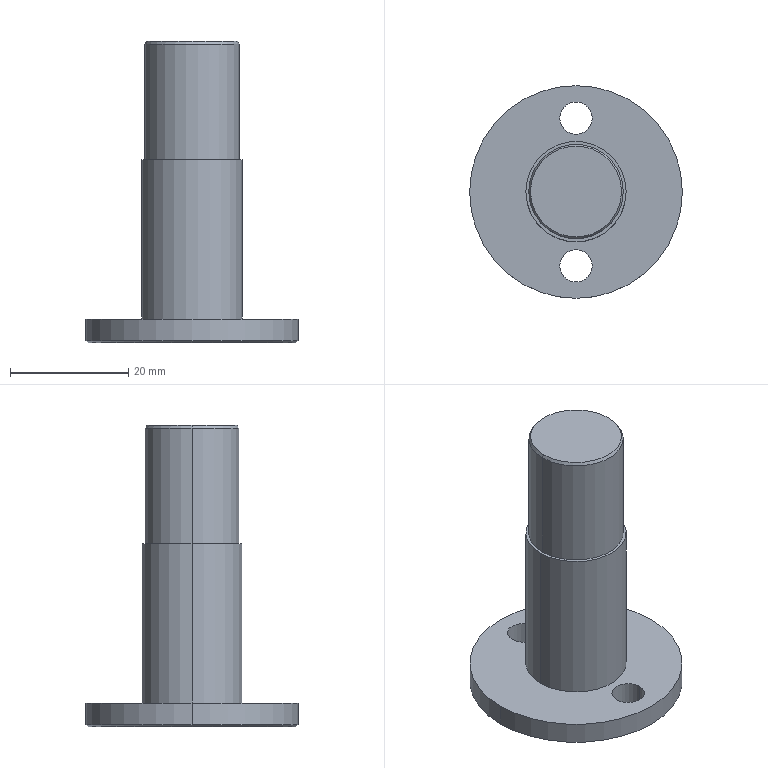Part | SolidWorks | features ICE 3, Chamfer 1, Extrusion 1 | 1 solid | 18 faces | box 36 x 36 x 51 mm | volume 14019 mm3 | cylinder 10 | cone 4 | plane 4 | commonest cylinder face diameters 5.5 x4 16 x2 17 x2 36 x2
STEP:
#1=CARTESIAN_POINT('',(-2.75,12.5,4.));
#2=VERTEX_POINT('',#1);
#3=CARTESIAN_POINT('',(2.75,12.5,4.));
#4=VERTEX_POINT('',#3);
#5=CARTESIAN_POINT('',(0.,12.5,4.));
#6=DIRECTION('',(0.,0.,1.));
#7=DIRECTION('',(1.,0.,0.));
#8=AXIS2_PLACEMENT_3D('',#5,#6,#7);
#9=CIRCLE('',#8,2.75);
#10=EDGE_CURVE('',#2,#4,#9,.T.);
#11=ORIENTED_EDGE('',*,*,#10,.T.);
#12=CARTESIAN_POINT('',(2.75,12.5,0.));
#13=VERTEX_POINT('',#12);
#14=CARTESIAN_POINT('',(2.75,12.5,20.));
#15=DIRECTION('',(0.,0.,-1.));
#16=VECTOR('',#15,1000.);
#17=LINE('',#14,#16);
#18=EDGE_CURVE('',#4,#13,#17,.T.);
#19=ORIENTED_EDGE('',*,*,#18,.T.);
#20=CARTESIAN_POINT('',(-2.75,12.5,0.));
#21=VERTEX_POINT('',#20);
#22=CARTESIAN_POINT('',(0.,12.5,0.));
#23=DIRECTION('',(0.,0.,-1.));
#24=DIRECTION('',(-1.,0.,0.));
#25=AXIS2_PLACEMENT_3D('',#22,#23,#24);
#26=CIRCLE('',#25,2.75);
#27=EDGE_CURVE('',#13,#21,#26,.T.);
#28=ORIENTED_EDGE('',*,*,#27,.T.);
#29=CARTESIAN_POINT('',(-2.75,12.5,20.));
#30=DIRECTION('',(0.,0.,-1.));
#31=VECTOR('',#30,1000.);
#32=LINE('',#29,#31);
#33=EDGE_CURVE('',#2,#21,#32,.T.);
#34=ORIENTED_EDGE('',*,*,#33,.F.);
#35=EDGE_LOOP('',(#11,#19,#28,#34));
#36=FACE_OUTER_BOUND('',#35,.T.);
#37=CARTESIAN_POINT('',(0.,12.5,20.));
#38=DIRECTION('',(0.,0.,-1.));
#39=DIRECTION('',(-1.,0.,0.));
#40=AXIS2_PLACEMENT_3D('',#37,#38,#39);
#41=CYLINDRICAL_SURFACE('',#40,2.75);
#42=ADVANCED_FACE('',(#36),#41,.F.);
#43=CARTESIAN_POINT('',(-2.75,-12.5,4.));
#44=VERTEX_POINT('',#43);
#45=CARTESIAN_POINT('',(2.75,-12.5,4.));
#46=VERTEX_POINT('',#45);
#47=CARTESIAN_POINT('',(0.,-12.5,4.));
#48=DIRECTION('',(0.,0.,1.));
#49=DIRECTION('',(1.,0.,0.));
#50=AXIS2_PLACEMENT_3D('',#47,#48,#49);
#51=CIRCLE('',#50,2.75);
#52=EDGE_CURVE('',#44,#46,#51,.T.);
#53=ORIENTED_EDGE('',*,*,#52,.T.);
#54=CARTESIAN_POINT('',(2.75,-12.5,0.));
#55=VERTEX_POINT('',#54);
#56=CARTESIAN_POINT('',(2.75,-12.5,20.));
#57=DIRECTION('',(0.,0.,-1.));
#58=VECTOR('',#57,1000.);
#59=LINE('',#56,#58);
#60=EDGE_CURVE('',#46,#55,#59,.T.);
#61=ORIENTED_EDGE('',*,*,#60,.T.);
#62=CARTESIAN_POINT('',(-2.75,-12.5,0.));
#63=VERTEX_POINT('',#62);
#64=CARTESIAN_POINT('',(0.,-12.5,0.));
#65=DIRECTION('',(0.,0.,-1.));
#66=DIRECTION('',(-1.,0.,0.));
#67=AXIS2_PLACEMENT_3D('',#64,#65,#66);
#68=CIRCLE('',#67,2.75);
#69=EDGE_CURVE('',#55,#63,#68,.T.);
#70=ORIENTED_EDGE('',*,*,#69,.T.);
#71=CARTESIAN_POINT('',(-2.75,-12.5,20.));
#72=DIRECTION('',(0.,0.,-1.));
#73=VECTOR('',#72,1000.);
#74=LINE('',#71,#73);
#75=EDGE_CURVE('',#44,#63,#74,.T.);
#76=ORIENTED_EDGE('',*,*,#75,.F.);
#77=EDGE_LOOP('',(#53,#61,#70,#76));
#78=FACE_OUTER_BOUND('',#77,.T.);
#79=CARTESIAN_POINT('',(0.,-12.5,20.));
#80=DIRECTION('',(0.,0.,-1.));
#81=DIRECTION('',(-1.,0.,0.));
#82=AXIS2_PLACEMENT_3D('',#79,#80,#81);
#83=CYLINDRICAL_SURFACE('',#82,2.75);
#84=ADVANCED_FACE('',(#78),#83,.F.);
#85=CARTESIAN_POINT('',(7.711,0.,51.));
#86=VERTEX_POINT('',#85);
#87=CARTESIAN_POINT('',(-7.711,0.,51.));
#88=VERTEX_POINT('',#87);
#89=CARTESIAN_POINT('',(0.,0.,51.));
#90=DIRECTION('',(0.,0.,1.));
#91=DIRECTION('',(1.,0.,0.));
#92=AXIS2_PLACEMENT_3D('',#89,#90,#91);
#93=CIRCLE('',#92,7.711);
#94=EDGE_CURVE('',#86,#88,#93,.T.);
#95=ORIENTED_EDGE('',*,*,#94,.F.);
#96=CARTESIAN_POINT('',(8.,0.,50.5));
#97=VERTEX_POINT('',#96);
#98=CARTESIAN_POINT('',(7.711,0.,51.));
#99=DIRECTION('',(0.5,0.,-0.866));
#100=VECTOR('',#99,1000.);
#101=LINE('',#98,#100);
#102=EDGE_CURVE('',#86,#97,#101,.T.);
#103=ORIENTED_EDGE('',*,*,#102,.T.);
#104=CARTESIAN_POINT('',(-8.,0.,50.5));
#105=VERTEX_POINT('',#104);
#106=CARTESIAN_POINT('',(0.,0.,50.5));
#107=DIRECTION('',(0.,0.,-1.));
#108=DIRECTION('',(1.,0.,0.));
#109=AXIS2_PLACEMENT_3D('',#106,#107,#108);
#110=CIRCLE('',#109,8.);
#111=EDGE_CURVE('',#105,#97,#110,.T.);
#112=ORIENTED_EDGE('',*,*,#111,.F.);
#113=CARTESIAN_POINT('',(-7.711,0.,51.));
#114=DIRECTION('',(-0.5,0.,-0.866));
#115=VECTOR('',#114,1000.);
#116=LINE('',#113,#115);
#117=EDGE_CURVE('',#88,#105,#116,.T.);
#118=ORIENTED_EDGE('',*,*,#117,.F.);
#119=EDGE_LOOP('',(#95,#103,#112,#118));
#120=FACE_OUTER_BOUND('',#119,.T.);
#121=CARTESIAN_POINT('',(0.,0.,51.));
#122=DIRECTION('',(0.,0.,-1.));
#123=DIRECTION('',(-1.,0.,0.));
#124=AXIS2_PLACEMENT_3D('',#121,#122,#123);
#125=CONICAL_SURFACE('',#124,7.711,0.5236);
#126=ADVANCED_FACE('',(#120),#125,.T.);
#127=CARTESIAN_POINT('',(-17.5,0.,0.));
#128=VERTEX_POINT('',#127);
#129=CARTESIAN_POINT('',(17.5,0.,0.));
#130=VERTEX_POINT('',#129);
#131=CARTESIAN_POINT('',(0.,0.,0.));
#132=DIRECTION('',(0.,0.,-1.));
#133=DIRECTION('',(1.,0.,0.));
#134=AXIS2_PLACEMENT_3D('',#131,#132,#133);
#135=CIRCLE('',#134,17.5);
#136=EDGE_CURVE('',#128,#130,#135,.T.);
#137=ORIENTED_EDGE('',*,*,#136,.F.);
#138=CARTESIAN_POINT('',(-18.,0.,0.2887));
#139=VERTEX_POINT('',#138);
#140=CARTESIAN_POINT('',(-18.,0.,0.2887));
#141=DIRECTION('',(-0.866,0.,0.5));
#142=VECTOR('',#141,1000.);
#143=LINE('',#140,#142);
#144=EDGE_CURVE('',#128,#139,#143,.T.);
#145=ORIENTED_EDGE('',*,*,#144,.T.);
#146=CARTESIAN_POINT('',(18.,0.,0.2887));
#147=VERTEX_POINT('',#146);
#148=CARTESIAN_POINT('',(0.,0.,0.2887));
#149=DIRECTION('',(0.,0.,1.));
#150=DIRECTION('',(1.,0.,0.));
#151=AXIS2_PLACEMENT_3D('',#148,#149,#150);
#152=CIRCLE('',#151,18.);
#153=EDGE_CURVE('',#147,#139,#152,.T.);
#154=ORIENTED_EDGE('',*,*,#153,.F.);
#155=CARTESIAN_POINT('',(18.,0.,0.2887));
#156=DIRECTION('',(0.866,0.,0.5));
#157=VECTOR('',#156,1000.);
#158=LINE('',#155,#157);
#159=EDGE_CURVE('',#130,#147,#158,.T.);
#160=ORIENTED_EDGE('',*,*,#159,.F.);
#161=EDGE_LOOP('',(#137,#145,#154,#160));
#162=FACE_OUTER_BOUND('',#161,.T.);
#163=CARTESIAN_POINT('',(0.,0.,0.2887));
#164=DIRECTION('',(0.,0.,1.));
#165=DIRECTION('',(1.,0.,0.));
#166=AXIS2_PLACEMENT_3D('',#163,#164,#165);
#167=CONICAL_SURFACE('',#166,18.,1.047);
#168=ADVANCED_FACE('',(#162),#167,.T.);
#169=ORIENTED_EDGE('',*,*,#111,.T.);
#170=CARTESIAN_POINT('',(8.,0.,31.));
#171=VERTEX_POINT('',#170);
#172=CARTESIAN_POINT('',(8.,0.,51.));
#173=DIRECTION('',(0.,0.,-1.));
#174=VECTOR('',#173,1000.);
#175=LINE('',#172,#174);
#176=EDGE_CURVE('',#97,#171,#175,.T.);
#177=ORIENTED_EDGE('',*,*,#176,.T.);
#178=CARTESIAN_POINT('',(-8.,0.,31.));
#179=VERTEX_POINT('',#178);
#180=CARTESIAN_POINT('',(0.,0.,31.));
#181=DIRECTION('',(0.,0.,1.));
#182=DIRECTION('',(1.,0.,0.));
#183=AXIS2_PLACEMENT_3D('',#180,#181,#182);
#184=CIRCLE('',#183,8.);
#185=EDGE_CURVE('',#171,#179,#184,.T.);
#186=ORIENTED_EDGE('',*,*,#185,.T.);
#187=CARTESIAN_POINT('',(-8.,0.,51.));
#188=DIRECTION('',(0.,0.,-1.));
#189=VECTOR('',#188,1000.);
#190=LINE('',#187,#189);
#191=EDGE_CURVE('',#105,#179,#190,.T.);
#192=ORIENTED_EDGE('',*,*,#191,.F.);
#193=EDGE_LOOP('',(#169,#177,#186,#192));
#194=FACE_OUTER_BOUND('',#193,.T.);
#195=CARTESIAN_POINT('',(0.,0.,51.));
#196=DIRECTION('',(0.,0.,-1.));
#197=DIRECTION('',(-1.,0.,0.));
#198=AXIS2_PLACEMENT_3D('',#195,#196,#197);
#199=CYLINDRICAL_SURFACE('',#198,8.);
#200=ADVANCED_FACE('',(#194),#199,.T.);
#201=CARTESIAN_POINT('',(8.5,0.,31.));
#202=VERTEX_POINT('',#201);
#203=CARTESIAN_POINT('',(-8.5,0.,31.));
#204=VERTEX_POINT('',#203);
#205=CARTESIAN_POINT('',(0.,0.,31.));
#206=DIRECTION('',(0.,0.,1.));
#207=DIRECTION('',(1.,0.,0.));
#208=AXIS2_PLACEMENT_3D('',#205,#206,#207);
#209=CIRCLE('',#208,8.5);
#210=EDGE_CURVE('',#202,#204,#209,.T.);
#211=ORIENTED_EDGE('',*,*,#210,.F.);
#212=CARTESIAN_POINT('',(8.5,0.,4.));
#213=VERTEX_POINT('',#212);
#214=CARTESIAN_POINT('',(8.5,0.,31.));
#215=DIRECTION('',(0.,0.,-1.));
#216=VECTOR('',#215,1000.);
#217=LINE('',#214,#216);
#218=EDGE_CURVE('',#202,#213,#217,.T.);
#219=ORIENTED_EDGE('',*,*,#218,.T.);
#220=CARTESIAN_POINT('',(-8.5,0.,4.));
#221=VERTEX_POINT('',#220);
#222=CARTESIAN_POINT('',(0.,0.,4.));
#223=DIRECTION('',(0.,0.,1.));
#224=DIRECTION('',(1.,0.,0.));
#225=AXIS2_PLACEMENT_3D('',#222,#223,#224);
#226=CIRCLE('',#225,8.5);
#227=EDGE_CURVE('',#213,#221,#226,.T.);
#228=ORIENTED_EDGE('',*,*,#227,.T.);
#229=CARTESIAN_POINT('',(-8.5,0.,31.));
#230=DIRECTION('',(0.,0.,-1.));
#231=VECTOR('',#230,1000.);
#232=LINE('',#229,#231);
#233=EDGE_CURVE('',#204,#221,#232,.T.);
#234=ORIENTED_EDGE('',*,*,#233,.F.);
#235=EDGE_LOOP('',(#211,#219,#228,#234));
#236=FACE_OUTER_BOUND('',#235,.T.);
#237=CARTESIAN_POINT('',(0.,0.,31.));
#238=DIRECTION('',(0.,0.,-1.));
#239=DIRECTION('',(-1.,0.,0.));
#240=AXIS2_PLACEMENT_3D('',#237,#238,#239);
#241=CYLINDRICAL_SURFACE('',#240,8.5);
#242=ADVANCED_FACE('',(#236),#241,.T.);
#243=CARTESIAN_POINT('',(18.,0.,4.));
#244=VERTEX_POINT('',#243);
#245=CARTESIAN_POINT('',(-18.,0.,4.));
#246=VERTEX_POINT('',#245);
#247=CARTESIAN_POINT('',(0.,0.,4.));
#248=DIRECTION('',(0.,0.,1.));
#249=DIRECTION('',(1.,0.,0.));
#250=AXIS2_PLACEMENT_3D('',#247,#248,#249);
#251=CIRCLE('',#250,18.);
#252=EDGE_CURVE('',#244,#246,#251,.T.);
#253=ORIENTED_EDGE('',*,*,#252,.F.);
#254=CARTESIAN_POINT('',(18.,0.,4.));
#255=DIRECTION('',(0.,0.,-1.));
#256=VECTOR('',#255,1000.);
#257=LINE('',#254,#256);
#258=EDGE_CURVE('',#244,#147,#257,.T.);
#259=ORIENTED_EDGE('',*,*,#258,.T.);
#260=ORIENTED_EDGE('',*,*,#153,.T.);
#261=CARTESIAN_POINT('',(-18.,0.,4.));
#262=DIRECTION('',(0.,0.,-1.));
#263=VECTOR('',#262,1000.);
#264=LINE('',#261,#263);
#265=EDGE_CURVE('',#246,#139,#264,.T.);
#266=ORIENTED_EDGE('',*,*,#265,.F.);
#267=EDGE_LOOP('',(#253,#259,#260,#266));
#268=FACE_OUTER_BOUND('',#267,.T.);
#269=CARTESIAN_POINT('',(0.,0.,4.));
#270=DIRECTION('',(0.,0.,-1.));
#271=DIRECTION('',(-1.,0.,0.));
#272=AXIS2_PLACEMENT_3D('',#269,#270,#271);
#273=CYLINDRICAL_SURFACE('',#272,18.);
#274=ADVANCED_FACE('',(#268),#273,.T.);
#275=ORIENTED_EDGE('',*,*,#258,.F.);
#276=CARTESIAN_POINT('',(0.,0.,4.));
#277=DIRECTION('',(0.,0.,1.));
#278=DIRECTION('',(1.,0.,0.));
#279=AXIS2_PLACEMENT_3D('',#276,#277,#278);
#280=CIRCLE('',#279,18.);
#281=EDGE_CURVE('',#246,#244,#280,.T.);
#282=ORIENTED_EDGE('',*,*,#281,.F.);
#283=ORIENTED_EDGE('',*,*,#265,.T.);
#284=CARTESIAN_POINT('',(0.,0.,0.2887));
#285=DIRECTION('',(0.,0.,1.));
#286=DIRECTION('',(1.,0.,0.));
#287=AXIS2_PLACEMENT_3D('',#284,#285,#286);
#288=CIRCLE('',#287,18.);
#289=EDGE_CURVE('',#139,#147,#288,.T.);
#290=ORIENTED_EDGE('',*,*,#289,.T.);
#291=EDGE_LOOP('',(#275,#282,#283,#290));
#292=FACE_OUTER_BOUND('',#291,.T.);
#293=CARTESIAN_POINT('',(0.,0.,4.));
#294=DIRECTION('',(0.,0.,-1.));
#295=DIRECTION('',(-1.,0.,0.));
#296=AXIS2_PLACEMENT_3D('',#293,#294,#295);
#297=CYLINDRICAL_SURFACE('',#296,18.);
#298=ADVANCED_FACE('',(#292),#297,.T.);
#299=ORIENTED_EDGE('',*,*,#10,.F.);
#300=CARTESIAN_POINT('',(0.,12.5,4.));
#301=DIRECTION('',(0.,0.,1.));
#302=DIRECTION('',(1.,0.,0.));
#303=AXIS2_PLACEMENT_3D('',#300,#301,#302);
#304=CIRCLE('',#303,2.75);
#305=EDGE_CURVE('',#4,#2,#304,.T.);
#306=ORIENTED_EDGE('',*,*,#305,.F.);
#307=EDGE_LOOP('',(#299,#306));
#308=FACE_BOUND('',#307,.T.);
#309=ORIENTED_EDGE('',*,*,#52,.F.);
#310=CARTESIAN_POINT('',(0.,-12.5,4.));
#311=DIRECTION('',(0.,0.,1.));
#312=DIRECTION('',(1.,0.,0.));
#313=AXIS2_PLACEMENT_3D('',#310,#311,#312);
#314=CIRCLE('',#313,2.75);
#315=EDGE_CURVE('',#46,#44,#314,.T.);
#316=ORIENTED_EDGE('',*,*,#315,.F.);
#317=EDGE_LOOP('',(#309,#316));
#318=FACE_BOUND('',#317,.T.);
#319=CARTESIAN_POINT('',(0.,0.,4.));
#320=DIRECTION('',(0.,0.,1.));
#321=DIRECTION('',(1.,0.,0.));
#322=AXIS2_PLACEMENT_3D('',#319,#320,#321);
#323=CIRCLE('',#322,8.5);
#324=EDGE_CURVE('',#221,#213,#323,.T.);
#325=ORIENTED_EDGE('',*,*,#324,.F.);
#326=ORIENTED_EDGE('',*,*,#227,.F.);
#327=EDGE_LOOP('',(#325,#326));
#328=FACE_BOUND('',#327,.T.);
#329=ORIENTED_EDGE('',*,*,#281,.T.);
#330=ORIENTED_EDGE('',*,*,#252,.T.);
#331=EDGE_LOOP('',(#329,#330));
#332=FACE_OUTER_BOUND('',#331,.T.);
#333=CARTESIAN_POINT('',(0.,0.,4.));
#334=DIRECTION('',(0.,0.,1.));
#335=DIRECTION('',(1.,0.,0.));
#336=AXIS2_PLACEMENT_3D('',#333,#334,#335);
#337=PLANE('',#336);
#338=ADVANCED_FACE('',(#308,#318,#328,#332),#337,.T.);
#339=CARTESIAN_POINT('',(0.,12.5,0.));
#340=DIRECTION('',(0.,0.,-1.));
#341=DIRECTION('',(-1.,0.,0.));
#342=AXIS2_PLACEMENT_3D('',#339,#340,#341);
#343=CIRCLE('',#342,2.75);
#344=EDGE_CURVE('',#21,#13,#343,.T.);
#345=ORIENTED_EDGE('',*,*,#344,.F.);
#346=ORIENTED_EDGE('',*,*,#27,.F.);
#347=EDGE_LOOP('',(#345,#346));
#348=FACE_BOUND('',#347,.T.);
#349=CARTESIAN_POINT('',(0.,-12.5,0.));
#350=DIRECTION('',(0.,0.,-1.));
#351=DIRECTION('',(-1.,0.,0.));
#352=AXIS2_PLACEMENT_3D('',#349,#350,#351);
#353=CIRCLE('',#352,2.75);
#354=EDGE_CURVE('',#63,#55,#353,.T.);
#355=ORIENTED_EDGE('',*,*,#354,.F.);
#356=ORIENTED_EDGE('',*,*,#69,.F.);
#357=EDGE_LOOP('',(#355,#356));
#358=FACE_BOUND('',#357,.T.);
#359=CARTESIAN_POINT('',(0.,0.,0.));
#360=DIRECTION('',(0.,0.,-1.));
#361=DIRECTION('',(1.,0.,0.));
#362=AXIS2_PLACEMENT_3D('',#359,#360,#361);
#363=CIRCLE('',#362,17.5);
#364=EDGE_CURVE('',#130,#128,#363,.T.);
#365=ORIENTED_EDGE('',*,*,#364,.T.);
#366=ORIENTED_EDGE('',*,*,#136,.T.);
#367=EDGE_LOOP('',(#365,#366));
#368=FACE_OUTER_BOUND('',#367,.T.);
#369=CARTESIAN_POINT('',(0.,0.,0.));
#370=DIRECTION('',(0.,0.,1.));
#371=DIRECTION('',(1.,0.,0.));
#372=AXIS2_PLACEMENT_3D('',#369,#370,#371);
#373=PLANE('',#372);
#374=ADVANCED_FACE('',(#348,#358,#368),#373,.F.);
#375=ORIENTED_EDGE('',*,*,#218,.F.);
#376=CARTESIAN_POINT('',(0.,0.,31.));
#377=DIRECTION('',(0.,0.,1.));
#378=DIRECTION('',(1.,0.,0.));
#379=AXIS2_PLACEMENT_3D('',#376,#377,#378);
#380=CIRCLE('',#379,8.5);
#381=EDGE_CURVE('',#204,#202,#380,.T.);
#382=ORIENTED_EDGE('',*,*,#381,.F.);
#383=ORIENTED_EDGE('',*,*,#233,.T.);
#384=ORIENTED_EDGE('',*,*,#324,.T.);
#385=EDGE_LOOP('',(#375,#382,#383,#384));
#386=FACE_OUTER_BOUND('',#385,.T.);
#387=CARTESIAN_POINT('',(0.,0.,31.));
#388=DIRECTION('',(0.,0.,-1.));
#389=DIRECTION('',(-1.,0.,0.));
#390=AXIS2_PLACEMENT_3D('',#387,#388,#389);
#391=CYLINDRICAL_SURFACE('',#390,8.5);
#392=ADVANCED_FACE('',(#386),#391,.T.);
#393=CARTESIAN_POINT('',(0.,0.,31.));
#394=DIRECTION('',(0.,0.,1.));
#395=DIRECTION('',(1.,0.,0.));
#396=AXIS2_PLACEMENT_3D('',#393,#394,#395);
#397=CIRCLE('',#396,8.);
#398=EDGE_CURVE('',#179,#171,#397,.T.);
#399=ORIENTED_EDGE('',*,*,#398,.F.);
#400=ORIENTED_EDGE('',*,*,#185,.F.);
#401=EDGE_LOOP('',(#399,#400));
#402=FACE_BOUND('',#401,.T.);
#403=ORIENTED_EDGE('',*,*,#381,.T.);
#404=ORIENTED_EDGE('',*,*,#210,.T.);
#405=EDGE_LOOP('',(#403,#404));
#406=FACE_OUTER_BOUND('',#405,.T.);
#407=CARTESIAN_POINT('',(0.,0.,31.));
#408=DIRECTION('',(0.,0.,1.));
#409=DIRECTION('',(1.,0.,0.));
#410=AXIS2_PLACEMENT_3D('',#407,#408,#409);
#411=PLANE('',#410);
#412=ADVANCED_FACE('',(#402,#406),#411,.T.);
#413=ORIENTED_EDGE('',*,*,#176,.F.);
#414=CARTESIAN_POINT('',(0.,0.,50.5));
#415=DIRECTION('',(0.,0.,-1.));
#416=DIRECTION('',(1.,0.,0.));
#417=AXIS2_PLACEMENT_3D('',#414,#415,#416);
#418=CIRCLE('',#417,8.);
#419=EDGE_CURVE('',#97,#105,#418,.T.);
#420=ORIENTED_EDGE('',*,*,#419,.T.);
#421=ORIENTED_EDGE('',*,*,#191,.T.);
#422=ORIENTED_EDGE('',*,*,#398,.T.);
#423=EDGE_LOOP('',(#413,#420,#421,#422));
#424=FACE_OUTER_BOUND('',#423,.T.);
#425=CARTESIAN_POINT('',(0.,0.,51.));
#426=DIRECTION('',(0.,0.,-1.));
#427=DIRECTION('',(-1.,0.,0.));
#428=AXIS2_PLACEMENT_3D('',#425,#426,#427);
#429=CYLINDRICAL_SURFACE('',#428,8.);
#430=ADVANCED_FACE('',(#424),#429,.T.);
#431=CARTESIAN_POINT('',(0.,0.,51.));
#432=DIRECTION('',(0.,0.,1.));
#433=DIRECTION('',(1.,0.,0.));
#434=AXIS2_PLACEMENT_3D('',#431,#432,#433);
#435=CIRCLE('',#434,7.711);
#436=EDGE_CURVE('',#88,#86,#435,.T.);
#437=ORIENTED_EDGE('',*,*,#436,.T.);
#438=ORIENTED_EDGE('',*,*,#94,.T.);
#439=EDGE_LOOP('',(#437,#438));
#440=FACE_OUTER_BOUND('',#439,.T.);
#441=CARTESIAN_POINT('',(0.,0.,51.));
#442=DIRECTION('',(0.,0.,1.));
#443=DIRECTION('',(1.,0.,0.));
#444=AXIS2_PLACEMENT_3D('',#441,#442,#443);
#445=PLANE('',#444);
#446=ADVANCED_FACE('',(#440),#445,.T.);
#447=ORIENTED_EDGE('',*,*,#144,.F.);
#448=ORIENTED_EDGE('',*,*,#364,.F.);
#449=ORIENTED_EDGE('',*,*,#159,.T.);
#450=ORIENTED_EDGE('',*,*,#289,.F.);
#451=EDGE_LOOP('',(#447,#448,#449,#450));
#452=FACE_OUTER_BOUND('',#451,.T.);
#453=CARTESIAN_POINT('',(0.,0.,0.2887));
#454=DIRECTION('',(0.,0.,1.));
#455=DIRECTION('',(1.,0.,0.));
#456=AXIS2_PLACEMENT_3D('',#453,#454,#455);
#457=CONICAL_SURFACE('',#456,18.,1.047);
#458=ADVANCED_FACE('',(#452),#457,.T.);
#459=ORIENTED_EDGE('',*,*,#102,.F.);
#460=ORIENTED_EDGE('',*,*,#436,.F.);
#461=ORIENTED_EDGE('',*,*,#117,.T.);
#462=ORIENTED_EDGE('',*,*,#419,.F.);
#463=EDGE_LOOP('',(#459,#460,#461,#462));
#464=FACE_OUTER_BOUND('',#463,.T.);
#465=CARTESIAN_POINT('',(0.,0.,51.));
#466=DIRECTION('',(0.,0.,-1.));
#467=DIRECTION('',(-1.,0.,0.));
#468=AXIS2_PLACEMENT_3D('',#465,#466,#467);
#469=CONICAL_SURFACE('',#468,7.711,0.5236);
#470=ADVANCED_FACE('',(#464),#469,.T.);
#471=ORIENTED_EDGE('',*,*,#60,.F.);
#472=ORIENTED_EDGE('',*,*,#315,.T.);
#473=ORIENTED_EDGE('',*,*,#75,.T.);
#474=ORIENTED_EDGE('',*,*,#354,.T.);
#475=EDGE_LOOP('',(#471,#472,#473,#474));
#476=FACE_OUTER_BOUND('',#475,.T.);
#477=CARTESIAN_POINT('',(0.,-12.5,20.));
#478=DIRECTION('',(0.,0.,-1.));
#479=DIRECTION('',(-1.,0.,0.));
#480=AXIS2_PLACEMENT_3D('',#477,#478,#479);
#481=CYLINDRICAL_SURFACE('',#480,2.75);
#482=ADVANCED_FACE('',(#476),#481,.F.);
#483=ORIENTED_EDGE('',*,*,#18,.F.);
#484=ORIENTED_EDGE('',*,*,#305,.T.);
#485=ORIENTED_EDGE('',*,*,#33,.T.);
#486=ORIENTED_EDGE('',*,*,#344,.T.);
#487=EDGE_LOOP('',(#483,#484,#485,#486));
#488=FACE_OUTER_BOUND('',#487,.T.);
#489=CARTESIAN_POINT('',(0.,12.5,20.));
#490=DIRECTION('',(0.,0.,-1.));
#491=DIRECTION('',(-1.,0.,0.));
#492=AXIS2_PLACEMENT_3D('',#489,#490,#491);
#493=CYLINDRICAL_SURFACE('',#492,2.75);
#494=ADVANCED_FACE('',(#488),#493,.F.);
#495=CLOSED_SHELL('',(#42,#84,#126,#168,#200,#242,#274,#298,#338,#374,#392,#412,#430,#446,#458,#470,#482,#494));
#496=MANIFOLD_SOLID_BREP('',#495);
#497=CARTESIAN_POINT('',(0.,0.,0.));
#498=DIRECTION('',(0.,0.,1.));
#499=DIRECTION('',(1.,0.,0.));
#500=AXIS2_PLACEMENT_3D('',#497,#498,#499);
#501=(LENGTH_UNIT()NAMED_UNIT(*)SI_UNIT(.MILLI.,.METRE.));
#502=UNCERTAINTY_MEASURE_WITH_UNIT(LENGTH_MEASURE(0.00001),#501,'','');
#503=(NAMED_UNIT(*)PLANE_ANGLE_UNIT()SI_UNIT($,.RADIAN.));
#504=(NAMED_UNIT(*)SI_UNIT($,.STERADIAN.)SOLID_ANGLE_UNIT());
#505=(GEOMETRIC_REPRESENTATION_CONTEXT(3)GLOBAL_UNCERTAINTY_ASSIGNED_CONTEXT((#502))GLOBAL_UNIT_ASSIGNED_CONTEXT((#501,#503,#504))REPRESENTATION_CONTEXT('',''));
#506=ADVANCED_BREP_SHAPE_REPRESENTATION('',(#496,#500),#505);